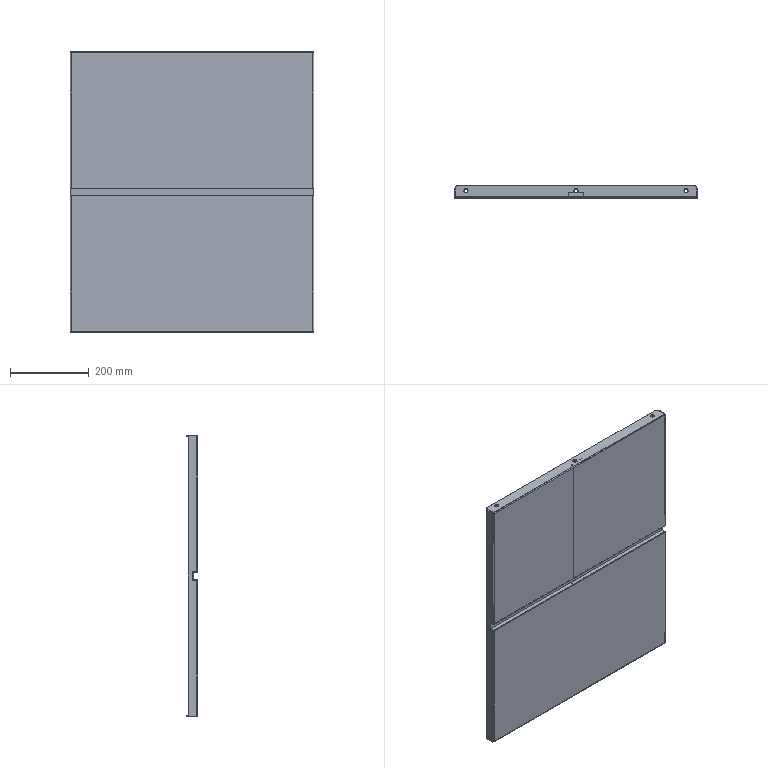Part | SolidWorks | features ICE 4, BossThin 2, Extrusion 1, Fillet 1, FlatPattern 1, FlattenBends 1, LPattern 1, ProcessBends 1, Rip 1, SheetMetal 1, Shell 1 | 4 solids | 118 faces | box 620 x 30 x 714 mm | volume 1123821 mm3 | plane 90 | cylinder 28 | commonest cylinder face diameters 10.5 x12 0.6 x6 4.6 x6 10 x4